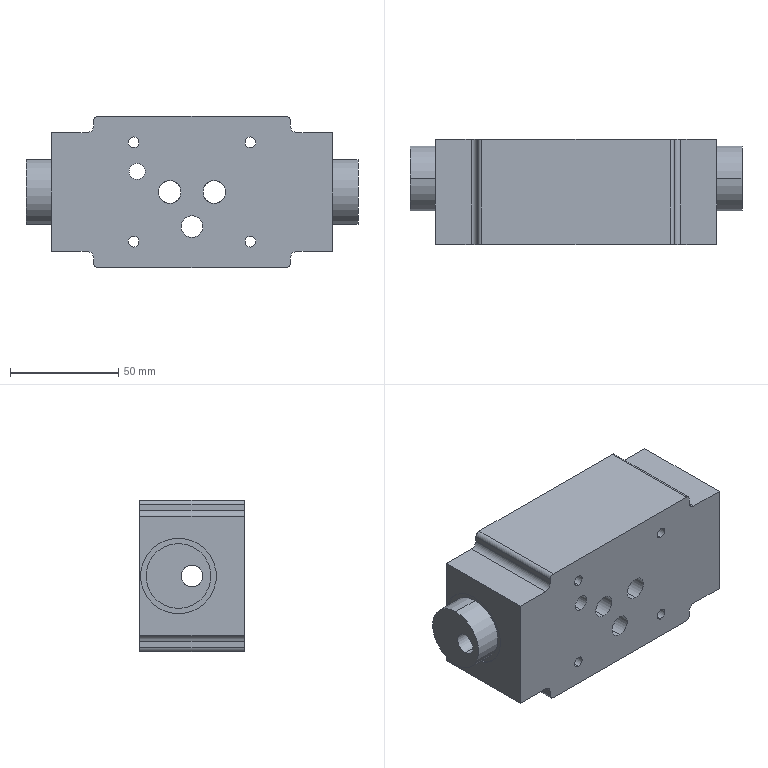Part | SolidWorks | features ICE 4, 3DProfileFeature 1, Extrusion 1, HoleWzd 1, MirrorPattern 1 | 1 solid | 56 faces | box 153.5 x 48.5 x 70 mm | volume 400500 mm3 | cylinder 38 | plane 18 | commonest cylinder face diameters 5 x8 10 x8 4 x4 6 x4 10.5 x4 30 x4